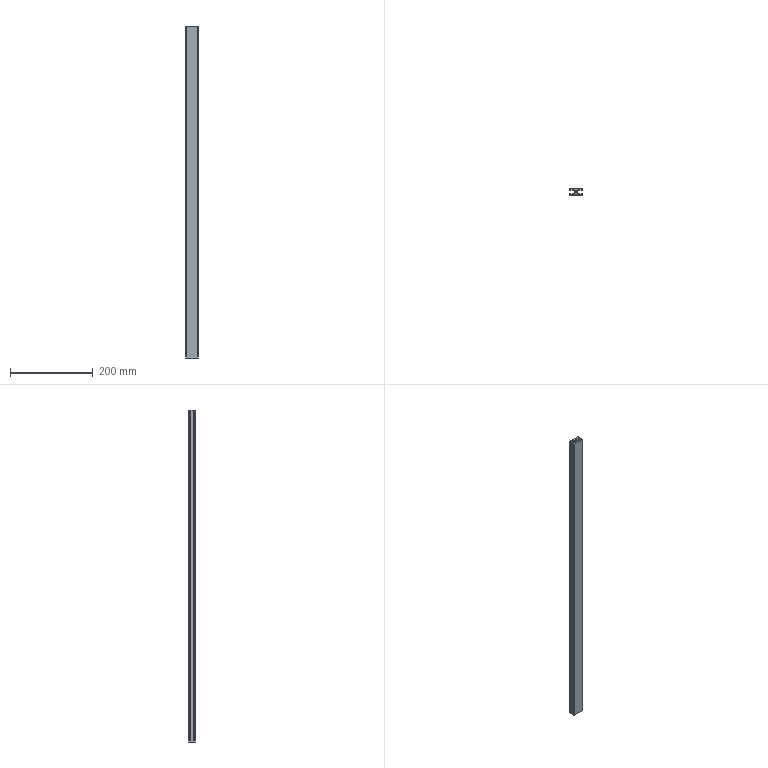Part | SolidWorks | features BaseBody 1, MoveFace 1 | 1 solid | 53 faces | box 30 x 15 x 802 mm | volume 193417 mm3 | plane 38 | cylinder 15 | commonest cylinder face diameters 1 x6 5 x5 2 x4